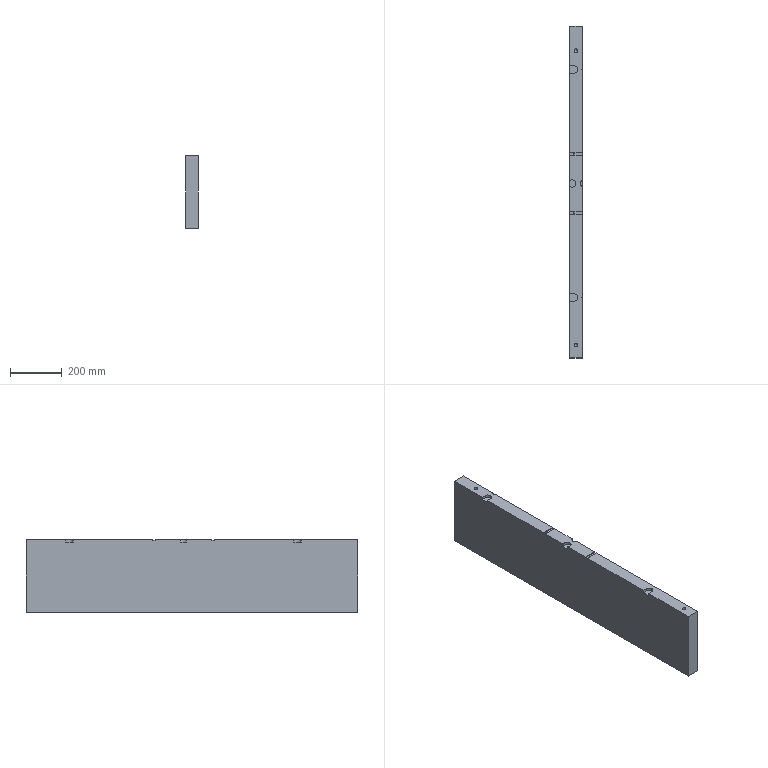Part | NX | features 29 2 | 1 solid | 44 faces | box 50 x 1280 x 280.5 mm | volume 17889049 mm3 | plane 24 | cylinder 13 | cone 7 | commonest cylinder face diameters 14.1 x5 28 x3 29 x3 3.4 x2
STEP:
#1=CARTESIAN_POINT('',(2892.05,512.5,-493.5));
#2=VERTEX_POINT('',#1);
#3=CARTESIAN_POINT('',(2885.,512.5,-493.5));
#4=DIRECTION('',(0.,0.,1.));
#5=DIRECTION('',(1.,0.,0.));
#6=AXIS2_PLACEMENT_3D('',#3,#4,#5);
#7=CIRCLE('',#6,7.05);
#8=EDGE_CURVE('',#2,#2,#7,.T.);
#9=ORIENTED_EDGE('',*,*,#8,.T.);
#10=EDGE_LOOP('',(#9));
#11=FACE_BOUND('',#10,.T.);
#12=CARTESIAN_POINT('',(2860.,607.5,-493.5));
#13=VERTEX_POINT('',#12);
#14=CARTESIAN_POINT('',(2860.,-672.5,-493.5));
#15=VERTEX_POINT('',#14);
#16=CARTESIAN_POINT('',(2860.,193.,-493.5));
#17=DIRECTION('',(0.,-1.,0.));
#18=VECTOR('',#17,1000.);
#19=LINE('',#16,#18);
#20=EDGE_CURVE('',#13,#15,#19,.T.);
#21=ORIENTED_EDGE('',*,*,#20,.F.);
#22=CARTESIAN_POINT('',(2910.,607.5,-493.5));
#23=VERTEX_POINT('',#22);
#24=CARTESIAN_POINT('',(2901.,607.5,-493.5));
#25=DIRECTION('',(1.,0.,0.));
#26=VECTOR('',#25,1000.);
#27=LINE('',#24,#26);
#28=EDGE_CURVE('',#13,#23,#27,.T.);
#29=ORIENTED_EDGE('',*,*,#28,.T.);
#30=CARTESIAN_POINT('',(2910.,-672.5,-493.5));
#31=VERTEX_POINT('',#30);
#32=CARTESIAN_POINT('',(2910.,193.,-493.5));
#33=DIRECTION('',(0.,1.,0.));
#34=VECTOR('',#33,1000.);
#35=LINE('',#32,#34);
#36=EDGE_CURVE('',#31,#23,#35,.T.);
#37=ORIENTED_EDGE('',*,*,#36,.F.);
#38=CARTESIAN_POINT('',(3250.,-672.5,-493.5));
#39=DIRECTION('',(-1.,0.,0.));
#40=VECTOR('',#39,1000.);
#41=LINE('',#38,#40);
#42=EDGE_CURVE('',#31,#15,#41,.T.);
#43=ORIENTED_EDGE('',*,*,#42,.T.);
#44=EDGE_LOOP('',(#21,#29,#37,#43));
#45=FACE_BOUND('',#44,.T.);
#46=CARTESIAN_POINT('',(2892.05,-622.5,-493.5));
#47=VERTEX_POINT('',#46);
#48=CARTESIAN_POINT('',(2885.,-622.5,-493.5));
#49=DIRECTION('',(0.,0.,1.));
#50=DIRECTION('',(1.,0.,0.));
#51=AXIS2_PLACEMENT_3D('',#48,#49,#50);
#52=CIRCLE('',#51,7.05);
#53=EDGE_CURVE('',#47,#47,#52,.T.);
#54=ORIENTED_EDGE('',*,*,#53,.T.);
#55=EDGE_LOOP('',(#54));
#56=FACE_BOUND('',#55,.T.);
#57=CARTESIAN_POINT('',(2892.05,-32.5,-493.5));
#58=VERTEX_POINT('',#57);
#59=CARTESIAN_POINT('',(2885.,-32.5,-493.5));
#60=DIRECTION('',(0.,0.,1.));
#61=DIRECTION('',(1.,0.,0.));
#62=AXIS2_PLACEMENT_3D('',#59,#60,#61);
#63=CIRCLE('',#62,7.05);
#64=EDGE_CURVE('',#58,#58,#63,.T.);
#65=ORIENTED_EDGE('',*,*,#64,.T.);
#66=EDGE_LOOP('',(#65));
#67=FACE_BOUND('',#66,.T.);
#68=CARTESIAN_POINT('',(1985.,0.,-493.5));
#69=DIRECTION('',(0.,0.,-1.));
#70=DIRECTION('',(1.,0.,0.));
#71=AXIS2_PLACEMENT_3D('',#68,#69,#70);
#72=PLANE('',#71);
#73=ADVANCED_FACE('',(#11,#45,#56,#67),#72,.T.);
#74=CARTESIAN_POINT('',(2910.,120.5,-213.));
#75=VERTEX_POINT('',#74);
#76=CARTESIAN_POINT('',(2860.,120.5,-213.));
#77=VERTEX_POINT('',#76);
#78=CARTESIAN_POINT('',(1985.,120.5,-213.));
#79=DIRECTION('',(-1.,0.,0.));
#80=VECTOR('',#79,1000.);
#81=LINE('',#78,#80);
#82=EDGE_CURVE('',#75,#77,#81,.T.);
#83=ORIENTED_EDGE('',*,*,#82,.F.);
#84=CARTESIAN_POINT('',(2910.,432.789,-213.));
#85=VERTEX_POINT('',#84);
#86=CARTESIAN_POINT('',(2910.,193.,-213.));
#87=DIRECTION('',(0.,-1.,0.));
#88=VECTOR('',#87,1000.);
#89=LINE('',#86,#88);
#90=EDGE_CURVE('',#85,#75,#89,.T.);
#91=ORIENTED_EDGE('',*,*,#90,.F.);
#92=CARTESIAN_POINT('',(2910.,447.211,-213.));
#93=VERTEX_POINT('',#92);
#94=CARTESIAN_POINT('',(2922.,440.,-213.));
#95=DIRECTION('',(0.,0.,1.));
#96=DIRECTION('',(-1.,0.,0.));
#97=AXIS2_PLACEMENT_3D('',#94,#95,#96);
#98=CIRCLE('',#97,14.);
#99=EDGE_CURVE('',#93,#85,#98,.T.);
#100=ORIENTED_EDGE('',*,*,#99,.F.);
#101=CARTESIAN_POINT('',(2910.,607.5,-213.));
#102=VERTEX_POINT('',#101);
#103=CARTESIAN_POINT('',(2910.,193.,-213.));
#104=DIRECTION('',(0.,-1.,0.));
#105=VECTOR('',#104,1000.);
#106=LINE('',#103,#105);
#107=EDGE_CURVE('',#102,#93,#106,.T.);
#108=ORIENTED_EDGE('',*,*,#107,.F.);
#109=CARTESIAN_POINT('',(2860.,607.5,-213.));
#110=VERTEX_POINT('',#109);
#111=CARTESIAN_POINT('',(2901.,607.5,-213.));
#112=DIRECTION('',(-1.,0.,0.));
#113=VECTOR('',#112,1000.);
#114=LINE('',#111,#113);
#115=EDGE_CURVE('',#102,#110,#114,.T.);
#116=ORIENTED_EDGE('',*,*,#115,.T.);
#117=CARTESIAN_POINT('',(2860.,454.5,-213.));
#118=VERTEX_POINT('',#117);
#119=CARTESIAN_POINT('',(2860.,193.,-213.));
#120=DIRECTION('',(0.,1.,0.));
#121=VECTOR('',#120,1000.);
#122=LINE('',#119,#121);
#123=EDGE_CURVE('',#118,#110,#122,.T.);
#124=ORIENTED_EDGE('',*,*,#123,.F.);
#125=CARTESIAN_POINT('',(2877.,454.5,-213.));
#126=VERTEX_POINT('',#125);
#127=CARTESIAN_POINT('',(1985.,454.5,-213.));
#128=DIRECTION('',(-1.,0.,0.));
#129=VECTOR('',#128,1000.);
#130=LINE('',#127,#129);
#131=EDGE_CURVE('',#126,#118,#130,.T.);
#132=ORIENTED_EDGE('',*,*,#131,.F.);
#133=CARTESIAN_POINT('',(2877.,425.5,-213.));
#134=VERTEX_POINT('',#133);
#135=CARTESIAN_POINT('',(2877.,440.,-213.));
#136=DIRECTION('',(0.,0.,1.));
#137=DIRECTION('',(-1.,0.,0.));
#138=AXIS2_PLACEMENT_3D('',#135,#136,#137);
#139=CIRCLE('',#138,14.5);
#140=EDGE_CURVE('',#134,#126,#139,.T.);
#141=ORIENTED_EDGE('',*,*,#140,.F.);
#142=CARTESIAN_POINT('',(2860.,425.5,-213.));
#143=VERTEX_POINT('',#142);
#144=CARTESIAN_POINT('',(1985.,425.5,-213.));
#145=DIRECTION('',(1.,0.,0.));
#146=VECTOR('',#145,1000.);
#147=LINE('',#144,#146);
#148=EDGE_CURVE('',#143,#134,#147,.T.);
#149=ORIENTED_EDGE('',*,*,#148,.F.);
#150=CARTESIAN_POINT('',(2860.,193.,-213.));
#151=DIRECTION('',(0.,1.,0.));
#152=VECTOR('',#151,1000.);
#153=LINE('',#150,#152);
#154=EDGE_CURVE('',#77,#143,#153,.T.);
#155=ORIENTED_EDGE('',*,*,#154,.F.);
#156=EDGE_LOOP('',(#83,#91,#100,#108,#116,#124,#132,#141,#149,#155));
#157=FACE_BOUND('',#156,.T.);
#158=CARTESIAN_POINT('',(2892.05,512.5,-213.));
#159=VERTEX_POINT('',#158);
#160=CARTESIAN_POINT('',(2885.,512.5,-213.));
#161=DIRECTION('',(0.,0.,-1.));
#162=DIRECTION('',(1.,0.,0.));
#163=AXIS2_PLACEMENT_3D('',#160,#161,#162);
#164=CIRCLE('',#163,7.05);
#165=EDGE_CURVE('',#159,#159,#164,.T.);
#166=ORIENTED_EDGE('',*,*,#165,.T.);
#167=EDGE_LOOP('',(#166));
#168=FACE_BOUND('',#167,.T.);
#169=CARTESIAN_POINT('',(1985.,0.,-213.));
#170=DIRECTION('',(0.,0.,1.));
#171=DIRECTION('',(-1.,0.,0.));
#172=AXIS2_PLACEMENT_3D('',#169,#170,#171);
#173=PLANE('',#172);
#174=ADVANCED_FACE('',(#157,#168),#173,.T.);
#175=CARTESIAN_POINT('',(2860.,-120.5,-213.));
#176=VERTEX_POINT('',#175);
#177=CARTESIAN_POINT('',(2910.,-120.5,-213.));
#178=VERTEX_POINT('',#177);
#179=CARTESIAN_POINT('',(1985.,-120.5,-213.));
#180=DIRECTION('',(1.,0.,0.));
#181=VECTOR('',#180,1000.);
#182=LINE('',#179,#181);
#183=EDGE_CURVE('',#176,#178,#182,.T.);
#184=ORIENTED_EDGE('',*,*,#183,.F.);
#185=CARTESIAN_POINT('',(2860.,-425.5,-213.));
#186=VERTEX_POINT('',#185);
#187=CARTESIAN_POINT('',(2860.,193.,-213.));
#188=DIRECTION('',(0.,1.,0.));
#189=VECTOR('',#188,1000.);
#190=LINE('',#187,#189);
#191=EDGE_CURVE('',#186,#176,#190,.T.);
#192=ORIENTED_EDGE('',*,*,#191,.F.);
#193=CARTESIAN_POINT('',(2877.,-425.5,-213.));
#194=VERTEX_POINT('',#193);
#195=CARTESIAN_POINT('',(1985.,-425.5,-213.));
#196=DIRECTION('',(-1.,0.,0.));
#197=VECTOR('',#196,1000.);
#198=LINE('',#195,#197);
#199=EDGE_CURVE('',#194,#186,#198,.T.);
#200=ORIENTED_EDGE('',*,*,#199,.F.);
#201=CARTESIAN_POINT('',(2877.,-454.5,-213.));
#202=VERTEX_POINT('',#201);
#203=CARTESIAN_POINT('',(2877.,-440.,-213.));
#204=DIRECTION('',(0.,0.,1.));
#205=DIRECTION('',(-1.,0.,0.));
#206=AXIS2_PLACEMENT_3D('',#203,#204,#205);
#207=CIRCLE('',#206,14.5);
#208=EDGE_CURVE('',#202,#194,#207,.T.);
#209=ORIENTED_EDGE('',*,*,#208,.F.);
#210=CARTESIAN_POINT('',(2860.,-454.5,-213.));
#211=VERTEX_POINT('',#210);
#212=CARTESIAN_POINT('',(1985.,-454.5,-213.));
#213=DIRECTION('',(1.,0.,0.));
#214=VECTOR('',#213,1000.);
#215=LINE('',#212,#214);
#216=EDGE_CURVE('',#211,#202,#215,.T.);
#217=ORIENTED_EDGE('',*,*,#216,.F.);
#218=CARTESIAN_POINT('',(2860.,-672.5,-213.));
#219=VERTEX_POINT('',#218);
#220=CARTESIAN_POINT('',(2860.,193.,-213.));
#221=DIRECTION('',(0.,1.,0.));
#222=VECTOR('',#221,1000.);
#223=LINE('',#220,#222);
#224=EDGE_CURVE('',#219,#211,#223,.T.);
#225=ORIENTED_EDGE('',*,*,#224,.F.);
#226=CARTESIAN_POINT('',(2910.,-672.5,-213.));
#227=VERTEX_POINT('',#226);
#228=CARTESIAN_POINT('',(3250.,-672.5,-213.));
#229=DIRECTION('',(1.,0.,0.));
#230=VECTOR('',#229,1000.);
#231=LINE('',#228,#230);
#232=EDGE_CURVE('',#219,#227,#231,.T.);
#233=ORIENTED_EDGE('',*,*,#232,.T.);
#234=CARTESIAN_POINT('',(2910.,-447.211,-213.));
#235=VERTEX_POINT('',#234);
#236=CARTESIAN_POINT('',(2910.,193.,-213.));
#237=DIRECTION('',(0.,-1.,0.));
#238=VECTOR('',#237,1000.);
#239=LINE('',#236,#238);
#240=EDGE_CURVE('',#235,#227,#239,.T.);
#241=ORIENTED_EDGE('',*,*,#240,.F.);
#242=CARTESIAN_POINT('',(2910.,-432.789,-213.));
#243=VERTEX_POINT('',#242);
#244=CARTESIAN_POINT('',(2922.,-440.,-213.));
#245=DIRECTION('',(0.,0.,1.));
#246=DIRECTION('',(-1.,0.,0.));
#247=AXIS2_PLACEMENT_3D('',#244,#245,#246);
#248=CIRCLE('',#247,14.);
#249=EDGE_CURVE('',#243,#235,#248,.T.);
#250=ORIENTED_EDGE('',*,*,#249,.F.);
#251=CARTESIAN_POINT('',(2910.,193.,-213.));
#252=DIRECTION('',(0.,-1.,0.));
#253=VECTOR('',#252,1000.);
#254=LINE('',#251,#253);
#255=EDGE_CURVE('',#178,#243,#254,.T.);
#256=ORIENTED_EDGE('',*,*,#255,.F.);
#257=EDGE_LOOP('',(#184,#192,#200,#209,#217,#225,#233,#241,#250,#256));
#258=FACE_BOUND('',#257,.T.);
#259=CARTESIAN_POINT('',(2892.05,-622.5,-213.));
#260=VERTEX_POINT('',#259);
#261=CARTESIAN_POINT('',(2885.,-622.5,-213.));
#262=DIRECTION('',(0.,0.,-1.));
#263=DIRECTION('',(1.,0.,0.));
#264=AXIS2_PLACEMENT_3D('',#261,#262,#263);
#265=CIRCLE('',#264,7.05);
#266=EDGE_CURVE('',#260,#260,#265,.T.);
#267=ORIENTED_EDGE('',*,*,#266,.T.);
#268=EDGE_LOOP('',(#267));
#269=FACE_BOUND('',#268,.T.);
#270=CARTESIAN_POINT('',(1985.,0.,-213.));
#271=DIRECTION('',(0.,0.,1.));
#272=DIRECTION('',(-1.,0.,0.));
#273=AXIS2_PLACEMENT_3D('',#270,#271,#272);
#274=PLANE('',#273);
#275=ADVANCED_FACE('',(#258,#269),#274,.T.);
#276=CARTESIAN_POINT('',(2910.,-109.5,-213.));
#277=VERTEX_POINT('',#276);
#278=CARTESIAN_POINT('',(2860.,-109.5,-213.));
#279=VERTEX_POINT('',#278);
#280=CARTESIAN_POINT('',(1985.,-109.5,-213.));
#281=DIRECTION('',(-1.,0.,0.));
#282=VECTOR('',#281,1000.);
#283=LINE('',#280,#282);
#284=EDGE_CURVE('',#277,#279,#283,.T.);
#285=ORIENTED_EDGE('',*,*,#284,.F.);
#286=CARTESIAN_POINT('',(2910.,-13.077,-213.));
#287=VERTEX_POINT('',#286);
#288=CARTESIAN_POINT('',(2910.,193.,-213.));
#289=DIRECTION('',(0.,-1.,0.));
#290=VECTOR('',#289,1000.);
#291=LINE('',#288,#290);
#292=EDGE_CURVE('',#287,#277,#291,.T.);
#293=ORIENTED_EDGE('',*,*,#292,.F.);
#294=CARTESIAN_POINT('',(2910.,13.077,-213.));
#295=VERTEX_POINT('',#294);
#296=CARTESIAN_POINT('',(2915.,0.,-213.));
#297=DIRECTION('',(0.,0.,1.));
#298=DIRECTION('',(-1.,0.,0.));
#299=AXIS2_PLACEMENT_3D('',#296,#297,#298);
#300=CIRCLE('',#299,14.);
#301=EDGE_CURVE('',#295,#287,#300,.T.);
#302=ORIENTED_EDGE('',*,*,#301,.F.);
#303=CARTESIAN_POINT('',(2910.,109.5,-213.));
#304=VERTEX_POINT('',#303);
#305=CARTESIAN_POINT('',(2910.,193.,-213.));
#306=DIRECTION('',(0.,-1.,0.));
#307=VECTOR('',#306,1000.);
#308=LINE('',#305,#307);
#309=EDGE_CURVE('',#304,#295,#308,.T.);
#310=ORIENTED_EDGE('',*,*,#309,.F.);
#311=CARTESIAN_POINT('',(2860.,109.5,-213.));
#312=VERTEX_POINT('',#311);
#313=CARTESIAN_POINT('',(1985.,109.5,-213.));
#314=DIRECTION('',(1.,0.,0.));
#315=VECTOR('',#314,1000.);
#316=LINE('',#313,#315);
#317=EDGE_CURVE('',#312,#304,#316,.T.);
#318=ORIENTED_EDGE('',*,*,#317,.F.);
#319=CARTESIAN_POINT('',(2860.,10.5,-213.));
#320=VERTEX_POINT('',#319);
#321=CARTESIAN_POINT('',(2860.,193.,-213.));
#322=DIRECTION('',(0.,1.,0.));
#323=VECTOR('',#322,1000.);
#324=LINE('',#321,#323);
#325=EDGE_CURVE('',#320,#312,#324,.T.);
#326=ORIENTED_EDGE('',*,*,#325,.F.);
#327=CARTESIAN_POINT('',(2860.,-10.5,-213.));
#328=VERTEX_POINT('',#327);
#329=CARTESIAN_POINT('',(2870.,0.,-213.));
#330=DIRECTION('',(0.,0.,-1.));
#331=DIRECTION('',(-1.,0.,0.));
#332=AXIS2_PLACEMENT_3D('',#329,#330,#331);
#333=CIRCLE('',#332,14.5);
#334=EDGE_CURVE('',#320,#328,#333,.T.);
#335=ORIENTED_EDGE('',*,*,#334,.T.);
#336=CARTESIAN_POINT('',(2860.,193.,-213.));
#337=DIRECTION('',(0.,1.,0.));
#338=VECTOR('',#337,1000.);
#339=LINE('',#336,#338);
#340=EDGE_CURVE('',#279,#328,#339,.T.);
#341=ORIENTED_EDGE('',*,*,#340,.F.);
#342=EDGE_LOOP('',(#285,#293,#302,#310,#318,#326,#335,#341));
#343=FACE_BOUND('',#342,.T.);
#344=CARTESIAN_POINT('',(1985.,0.,-213.));
#345=DIRECTION('',(0.,0.,1.));
#346=DIRECTION('',(-1.,0.,0.));
#347=AXIS2_PLACEMENT_3D('',#344,#345,#346);
#348=PLANE('',#347);
#349=ADVANCED_FACE('',(#343),#348,.T.);
#350=CARTESIAN_POINT('',(2877.,425.5,-223.));
#351=VERTEX_POINT('',#350);
#352=CARTESIAN_POINT('',(2877.,425.5,-193.));
#353=DIRECTION('',(0.,0.,-1.));
#354=VECTOR('',#353,1000.);
#355=LINE('',#352,#354);
#356=EDGE_CURVE('',#134,#351,#355,.T.);
#357=ORIENTED_EDGE('',*,*,#356,.F.);
#358=ORIENTED_EDGE('',*,*,#140,.T.);
#359=CARTESIAN_POINT('',(2877.,454.5,-223.));
#360=VERTEX_POINT('',#359);
#361=CARTESIAN_POINT('',(2877.,454.5,-193.));
#362=DIRECTION('',(0.,0.,1.));
#363=VECTOR('',#362,1000.);
#364=LINE('',#361,#363);
#365=EDGE_CURVE('',#360,#126,#364,.T.);
#366=ORIENTED_EDGE('',*,*,#365,.F.);
#367=CARTESIAN_POINT('',(2877.,440.,-223.));
#368=DIRECTION('',(0.,0.,-1.));
#369=DIRECTION('',(-1.,0.,0.));
#370=AXIS2_PLACEMENT_3D('',#367,#368,#369);
#371=CIRCLE('',#370,14.5);
#372=EDGE_CURVE('',#360,#351,#371,.T.);
#373=ORIENTED_EDGE('',*,*,#372,.T.);
#374=EDGE_LOOP('',(#357,#358,#366,#373));
#375=FACE_BOUND('',#374,.T.);
#376=CARTESIAN_POINT('',(2877.,440.,-223.));
#377=DIRECTION('',(0.,0.,1.));
#378=DIRECTION('',(-1.,0.,0.));
#379=AXIS2_PLACEMENT_3D('',#376,#377,#378);
#380=CYLINDRICAL_SURFACE('',#379,14.5);
#381=ADVANCED_FACE('',(#375),#380,.F.);
#382=CARTESIAN_POINT('',(2877.,-454.5,-223.));
#383=VERTEX_POINT('',#382);
#384=CARTESIAN_POINT('',(2877.,-454.5,-193.));
#385=DIRECTION('',(0.,0.,-1.));
#386=VECTOR('',#385,1000.);
#387=LINE('',#384,#386);
#388=EDGE_CURVE('',#202,#383,#387,.T.);
#389=ORIENTED_EDGE('',*,*,#388,.F.);
#390=ORIENTED_EDGE('',*,*,#208,.T.);
#391=CARTESIAN_POINT('',(2877.,-425.5,-223.));
#392=VERTEX_POINT('',#391);
#393=CARTESIAN_POINT('',(2877.,-425.5,-193.));
#394=DIRECTION('',(0.,0.,1.));
#395=VECTOR('',#394,1000.);
#396=LINE('',#393,#395);
#397=EDGE_CURVE('',#392,#194,#396,.T.);
#398=ORIENTED_EDGE('',*,*,#397,.F.);
#399=CARTESIAN_POINT('',(2877.,-440.,-223.));
#400=DIRECTION('',(0.,0.,-1.));
#401=DIRECTION('',(-1.,0.,0.));
#402=AXIS2_PLACEMENT_3D('',#399,#400,#401);
#403=CIRCLE('',#402,14.5);
#404=EDGE_CURVE('',#392,#383,#403,.T.);
#405=ORIENTED_EDGE('',*,*,#404,.T.);
#406=EDGE_LOOP('',(#389,#390,#398,#405));
#407=FACE_BOUND('',#406,.T.);
#408=CARTESIAN_POINT('',(2877.,-440.,-223.));
#409=DIRECTION('',(0.,0.,1.));
#410=DIRECTION('',(-1.,0.,0.));
#411=AXIS2_PLACEMENT_3D('',#408,#409,#410);
#412=CYLINDRICAL_SURFACE('',#411,14.5);
#413=ADVANCED_FACE('',(#407),#412,.F.);
#414=CARTESIAN_POINT('',(2860.,-109.5,-216.));
#415=VERTEX_POINT('',#414);
#416=CARTESIAN_POINT('',(2860.,-109.5,-205.5));
#417=DIRECTION('',(0.,0.,-1.));
#418=VECTOR('',#417,1000.);
#419=LINE('',#416,#418);
#420=EDGE_CURVE('',#279,#415,#419,.T.);
#421=ORIENTED_EDGE('',*,*,#420,.F.);
#422=ORIENTED_EDGE('',*,*,#340,.T.);
#423=CARTESIAN_POINT('',(2860.,-10.5,-223.));
#424=VERTEX_POINT('',#423);
#425=CARTESIAN_POINT('',(2860.,-10.5,-223.));
#426=DIRECTION('',(0.,0.,-1.));
#427=VECTOR('',#426,1000.);
#428=LINE('',#425,#427);
#429=EDGE_CURVE('',#328,#424,#428,.T.);
#430=ORIENTED_EDGE('',*,*,#429,.T.);
#431=CARTESIAN_POINT('',(2860.,10.5,-223.));
#432=VERTEX_POINT('',#431);
#433=CARTESIAN_POINT('',(2860.,193.,-223.));
#434=DIRECTION('',(0.,-1.,0.));
#435=VECTOR('',#434,1000.);
#436=LINE('',#433,#435);
#437=EDGE_CURVE('',#432,#424,#436,.T.);
#438=ORIENTED_EDGE('',*,*,#437,.F.);
#439=CARTESIAN_POINT('',(2860.,10.5,-223.));
#440=DIRECTION('',(0.,0.,1.));
#441=VECTOR('',#440,1000.);
#442=LINE('',#439,#441);
#443=EDGE_CURVE('',#432,#320,#442,.T.);
#444=ORIENTED_EDGE('',*,*,#443,.T.);
#445=ORIENTED_EDGE('',*,*,#325,.T.);
#446=CARTESIAN_POINT('',(2860.,109.5,-216.));
#447=VERTEX_POINT('',#446);
#448=CARTESIAN_POINT('',(2860.,109.5,-205.5));
#449=DIRECTION('',(0.,0.,1.));
#450=VECTOR('',#449,1000.);
#451=LINE('',#448,#450);
#452=EDGE_CURVE('',#447,#312,#451,.T.);
#453=ORIENTED_EDGE('',*,*,#452,.F.);
#454=CARTESIAN_POINT('',(2860.,120.5,-216.));
#455=VERTEX_POINT('',#454);
#456=CARTESIAN_POINT('',(2860.,193.,-216.));
#457=DIRECTION('',(0.,-1.,0.));
#458=VECTOR('',#457,1000.);
#459=LINE('',#456,#458);
#460=EDGE_CURVE('',#455,#447,#459,.T.);
#461=ORIENTED_EDGE('',*,*,#460,.F.);
#462=CARTESIAN_POINT('',(2860.,120.5,-205.5));
#463=DIRECTION('',(0.,0.,-1.));
#464=VECTOR('',#463,1000.);
#465=LINE('',#462,#464);
#466=EDGE_CURVE('',#77,#455,#465,.T.);
#467=ORIENTED_EDGE('',*,*,#466,.F.);
#468=ORIENTED_EDGE('',*,*,#154,.T.);
#469=CARTESIAN_POINT('',(2860.,425.5,-223.));
#470=VERTEX_POINT('',#469);
#471=CARTESIAN_POINT('',(2860.,425.5,-205.5));
#472=DIRECTION('',(0.,0.,1.));
#473=VECTOR('',#472,1000.);
#474=LINE('',#471,#473);
#475=EDGE_CURVE('',#470,#143,#474,.T.);
#476=ORIENTED_EDGE('',*,*,#475,.F.);
#477=CARTESIAN_POINT('',(2860.,454.5,-223.));
#478=VERTEX_POINT('',#477);
#479=CARTESIAN_POINT('',(2860.,193.,-223.));
#480=DIRECTION('',(0.,1.,0.));
#481=VECTOR('',#480,1000.);
#482=LINE('',#479,#481);
#483=EDGE_CURVE('',#470,#478,#482,.T.);
#484=ORIENTED_EDGE('',*,*,#483,.T.);
#485=CARTESIAN_POINT('',(2860.,454.5,-205.5));
#486=DIRECTION('',(0.,0.,-1.));
#487=VECTOR('',#486,1000.);
#488=LINE('',#485,#487);
#489=EDGE_CURVE('',#118,#478,#488,.T.);
#490=ORIENTED_EDGE('',*,*,#489,.F.);
#491=ORIENTED_EDGE('',*,*,#123,.T.);
#492=CARTESIAN_POINT('',(2860.,607.5,-205.5));
#493=DIRECTION('',(0.,0.,1.));
#494=VECTOR('',#493,1000.);
#495=LINE('',#492,#494);
#496=EDGE_CURVE('',#13,#110,#495,.T.);
#497=ORIENTED_EDGE('',*,*,#496,.F.);
#498=ORIENTED_EDGE('',*,*,#20,.T.);
#499=CARTESIAN_POINT('',(2860.,-672.5,-113.));
#500=DIRECTION('',(0.,0.,1.));
#501=VECTOR('',#500,1000.);
#502=LINE('',#499,#501);
#503=EDGE_CURVE('',#15,#219,#502,.T.);
#504=ORIENTED_EDGE('',*,*,#503,.T.);
#505=ORIENTED_EDGE('',*,*,#224,.T.);
#506=CARTESIAN_POINT('',(2860.,-454.5,-223.));
#507=VERTEX_POINT('',#506);
#508=CARTESIAN_POINT('',(2860.,-454.5,-205.5));
#509=DIRECTION('',(0.,0.,1.));
#510=VECTOR('',#509,1000.);
#511=LINE('',#508,#510);
#512=EDGE_CURVE('',#507,#211,#511,.T.);
#513=ORIENTED_EDGE('',*,*,#512,.F.);
#514=CARTESIAN_POINT('',(2860.,-425.5,-223.));
#515=VERTEX_POINT('',#514);
#516=CARTESIAN_POINT('',(2860.,193.,-223.));
#517=DIRECTION('',(0.,1.,0.));
#518=VECTOR('',#517,1000.);
#519=LINE('',#516,#518);
#520=EDGE_CURVE('',#507,#515,#519,.T.);
#521=ORIENTED_EDGE('',*,*,#520,.T.);
#522=CARTESIAN_POINT('',(2860.,-425.5,-205.5));
#523=DIRECTION('',(0.,0.,-1.));
#524=VECTOR('',#523,1000.);
#525=LINE('',#522,#524);
#526=EDGE_CURVE('',#186,#515,#525,.T.);
#527=ORIENTED_EDGE('',*,*,#526,.F.);
#528=ORIENTED_EDGE('',*,*,#191,.T.);
#529=CARTESIAN_POINT('',(2860.,-120.5,-216.));
#530=VERTEX_POINT('',#529);
#531=CARTESIAN_POINT('',(2860.,-120.5,-205.5));
#532=DIRECTION('',(0.,0.,1.));
#533=VECTOR('',#532,1000.);
#534=LINE('',#531,#533);
#535=EDGE_CURVE('',#530,#176,#534,.T.);
#536=ORIENTED_EDGE('',*,*,#535,.F.);
#537=CARTESIAN_POINT('',(2860.,193.,-216.));
#538=DIRECTION('',(0.,-1.,0.));
#539=VECTOR('',#538,1000.);
#540=LINE('',#537,#539);
#541=EDGE_CURVE('',#415,#530,#540,.T.);
#542=ORIENTED_EDGE('',*,*,#541,.F.);
#543=EDGE_LOOP('',(#421,#422,#430,#438,#444,#445,#453,#461,#467,#468,#476,#484,#490,#491,#497,#498,#504,#505,#513,#521,#527,#528,#536,#542));
#544=FACE_BOUND('',#543,.T.);
#545=CARTESIAN_POINT('',(2860.,193.,-205.5));
#546=DIRECTION('',(-1.,0.,0.));
#547=DIRECTION('',(0.,0.,1.));
#548=AXIS2_PLACEMENT_3D('',#545,#546,#547);
#549=PLANE('',#548);
#550=ADVANCED_FACE('',(#544),#549,.T.);
#551=ORIENTED_EDGE('',*,*,#28,.F.);
#552=ORIENTED_EDGE('',*,*,#496,.T.);
#553=ORIENTED_EDGE('',*,*,#115,.F.);
#554=CARTESIAN_POINT('',(2910.,607.5,-339.));
#555=DIRECTION('',(0.,0.,1.));
#556=VECTOR('',#555,1000.);
#557=LINE('',#554,#556);
#558=EDGE_CURVE('',#23,#102,#557,.T.);
#559=ORIENTED_EDGE('',*,*,#558,.F.);
#560=EDGE_LOOP('',(#551,#552,#553,#559));
#561=FACE_BOUND('',#560,.T.);
#562=CARTESIAN_POINT('',(2901.,607.5,-339.));
#563=DIRECTION('',(0.,1.,0.));
#564=DIRECTION('',(1.,0.,0.));
#565=AXIS2_PLACEMENT_3D('',#562,#563,#564);
#566=PLANE('',#565);
#567=ADVANCED_FACE('',(#561),#566,.T.);
#568=CARTESIAN_POINT('',(2910.,-109.5,-216.));
#569=VERTEX_POINT('',#568);
#570=CARTESIAN_POINT('',(2910.,-109.5,-205.5));
#571=DIRECTION('',(0.,0.,1.));
#572=VECTOR('',#571,1000.);
#573=LINE('',#570,#572);
#574=EDGE_CURVE('',#569,#277,#573,.T.);
#575=ORIENTED_EDGE('',*,*,#574,.F.);
#576=CARTESIAN_POINT('',(2910.,-120.5,-216.));
#577=VERTEX_POINT('',#576);
#578=CARTESIAN_POINT('',(2910.,193.,-216.));
#579=DIRECTION('',(0.,1.,0.));
#580=VECTOR('',#579,1000.);
#581=LINE('',#578,#580);
#582=EDGE_CURVE('',#577,#569,#581,.T.);
#583=ORIENTED_EDGE('',*,*,#582,.F.);
#584=CARTESIAN_POINT('',(2910.,-120.5,-205.5));
#585=DIRECTION('',(0.,0.,-1.));
#586=VECTOR('',#585,1000.);
#587=LINE('',#584,#586);
#588=EDGE_CURVE('',#178,#577,#587,.T.);
#589=ORIENTED_EDGE('',*,*,#588,.F.);
#590=ORIENTED_EDGE('',*,*,#255,.T.);
#591=CARTESIAN_POINT('',(2910.,-432.789,-243.));
#592=VERTEX_POINT('',#591);
#593=CARTESIAN_POINT('',(2910.,-432.789,-243.));
#594=DIRECTION('',(0.,0.,1.));
#595=VECTOR('',#594,1000.);
#596=LINE('',#593,#595);
#597=EDGE_CURVE('',#592,#243,#596,.T.);
#598=ORIENTED_EDGE('',*,*,#597,.F.);
#599=CARTESIAN_POINT('',(2910.,-447.211,-243.));
#600=VERTEX_POINT('',#599);
#601=CARTESIAN_POINT('',(2910.,193.,-243.));
#602=DIRECTION('',(0.,-1.,0.));
#603=VECTOR('',#602,1000.);
#604=LINE('',#601,#603);
#605=EDGE_CURVE('',#592,#600,#604,.T.);
#606=ORIENTED_EDGE('',*,*,#605,.T.);
#607=CARTESIAN_POINT('',(2910.,-447.211,-243.));
#608=DIRECTION('',(0.,0.,-1.));
#609=VECTOR('',#608,1000.);
#610=LINE('',#607,#609);
#611=EDGE_CURVE('',#235,#600,#610,.T.);
#612=ORIENTED_EDGE('',*,*,#611,.F.);
#613=ORIENTED_EDGE('',*,*,#240,.T.);
#614=CARTESIAN_POINT('',(2910.,-672.5,-543.5));
#615=DIRECTION('',(0.,0.,1.));
#616=VECTOR('',#615,1000.);
#617=LINE('',#614,#616);
#618=EDGE_CURVE('',#31,#227,#617,.T.);
#619=ORIENTED_EDGE('',*,*,#618,.F.);
#620=ORIENTED_EDGE('',*,*,#36,.T.);
#621=ORIENTED_EDGE('',*,*,#558,.T.);
#622=ORIENTED_EDGE('',*,*,#107,.T.);
#623=CARTESIAN_POINT('',(2910.,447.211,-243.));
#624=VERTEX_POINT('',#623);
#625=CARTESIAN_POINT('',(2910.,447.211,-243.));
#626=DIRECTION('',(0.,0.,1.));
#627=VECTOR('',#626,1000.);
#628=LINE('',#625,#627);
#629=EDGE_CURVE('',#624,#93,#628,.T.);
#630=ORIENTED_EDGE('',*,*,#629,.F.);
#631=CARTESIAN_POINT('',(2910.,432.789,-243.));
#632=VERTEX_POINT('',#631);
#633=CARTESIAN_POINT('',(2910.,193.,-243.));
#634=DIRECTION('',(0.,-1.,0.));
#635=VECTOR('',#634,1000.);
#636=LINE('',#633,#635);
#637=EDGE_CURVE('',#624,#632,#636,.T.);
#638=ORIENTED_EDGE('',*,*,#637,.T.);
#639=CARTESIAN_POINT('',(2910.,432.789,-243.));
#640=DIRECTION('',(0.,0.,-1.));
#641=VECTOR('',#640,1000.);
#642=LINE('',#639,#641);
#643=EDGE_CURVE('',#85,#632,#642,.T.);
#644=ORIENTED_EDGE('',*,*,#643,.F.);
#645=ORIENTED_EDGE('',*,*,#90,.T.);
#646=CARTESIAN_POINT('',(2910.,120.5,-216.));
#647=VERTEX_POINT('',#646);
#648=CARTESIAN_POINT('',(2910.,120.5,-205.5));
#649=DIRECTION('',(0.,0.,1.));
#650=VECTOR('',#649,1000.);
#651=LINE('',#648,#650);
#652=EDGE_CURVE('',#647,#75,#651,.T.);
#653=ORIENTED_EDGE('',*,*,#652,.F.);
#654=CARTESIAN_POINT('',(2910.,109.5,-216.));
#655=VERTEX_POINT('',#654);
#656=CARTESIAN_POINT('',(2910.,193.,-216.));
#657=DIRECTION('',(0.,1.,0.));
#658=VECTOR('',#657,1000.);
#659=LINE('',#656,#658);
#660=EDGE_CURVE('',#655,#647,#659,.T.);
#661=ORIENTED_EDGE('',*,*,#660,.F.);
#662=CARTESIAN_POINT('',(2910.,109.5,-205.5));
#663=DIRECTION('',(0.,0.,-1.));
#664=VECTOR('',#663,1000.);
#665=LINE('',#662,#664);
#666=EDGE_CURVE('',#304,#655,#665,.T.);
#667=ORIENTED_EDGE('',*,*,#666,.F.);
#668=ORIENTED_EDGE('',*,*,#309,.T.);
#669=CARTESIAN_POINT('',(2910.,13.077,-243.));
#670=VERTEX_POINT('',#669);
#671=CARTESIAN_POINT('',(2910.,13.077,-243.));
#672=DIRECTION('',(0.,0.,1.));
#673=VECTOR('',#672,1000.);
#674=LINE('',#671,#673);
#675=EDGE_CURVE('',#670,#295,#674,.T.);
#676=ORIENTED_EDGE('',*,*,#675,.F.);
#677=CARTESIAN_POINT('',(2910.,-13.077,-243.));
#678=VERTEX_POINT('',#677);
#679=CARTESIAN_POINT('',(2910.,193.,-243.));
#680=DIRECTION('',(0.,-1.,0.));
#681=VECTOR('',#680,1000.);
#682=LINE('',#679,#681);
#683=EDGE_CURVE('',#670,#678,#682,.T.);
#684=ORIENTED_EDGE('',*,*,#683,.T.);
#685=CARTESIAN_POINT('',(2910.,-13.077,-243.));
#686=DIRECTION('',(0.,0.,-1.));
#687=VECTOR('',#686,1000.);
#688=LINE('',#685,#687);
#689=EDGE_CURVE('',#287,#678,#688,.T.);
#690=ORIENTED_EDGE('',*,*,#689,.F.);
#691=ORIENTED_EDGE('',*,*,#292,.T.);
#692=EDGE_LOOP('',(#575,#583,#589,#590,#598,#606,#612,#613,#619,#620,#621,#622,#630,#638,#644,#645,#653,#661,#667,#668,#676,#684,#690,#691));
#693=FACE_BOUND('',#692,.T.);
#694=CARTESIAN_POINT('',(2910.,193.,-205.5));
#695=DIRECTION('',(1.,0.,0.));
#696=DIRECTION('',(0.,0.,-1.));
#697=AXIS2_PLACEMENT_3D('',#694,#695,#696);
#698=PLANE('',#697);
#699=ADVANCED_FACE('',(#693),#698,.T.);
#700=ORIENTED_EDGE('',*,*,#42,.F.);
#701=ORIENTED_EDGE('',*,*,#618,.T.);
#702=ORIENTED_EDGE('',*,*,#232,.F.);
#703=ORIENTED_EDGE('',*,*,#503,.F.);
#704=EDGE_LOOP('',(#700,#701,#702,#703));
#705=FACE_BOUND('',#704,.T.);
#706=CARTESIAN_POINT('',(3250.,-672.5,-113.));
#707=DIRECTION('',(0.,1.,0.));
#708=DIRECTION('',(1.,0.,0.));
#709=AXIS2_PLACEMENT_3D('',#706,#707,#708);
#710=PLANE('',#709);
#711=ADVANCED_FACE('',(#705),#710,.F.);
#712=ORIENTED_EDGE('',*,*,#597,.T.);
#713=ORIENTED_EDGE('',*,*,#249,.T.);
#714=ORIENTED_EDGE('',*,*,#611,.T.);
#715=CARTESIAN_POINT('',(2922.,-440.,-243.));
#716=DIRECTION('',(0.,0.,-1.));
#717=DIRECTION('',(-1.,0.,0.));
#718=AXIS2_PLACEMENT_3D('',#715,#716,#717);
#719=CIRCLE('',#718,14.);
#720=EDGE_CURVE('',#600,#592,#719,.T.);
#721=ORIENTED_EDGE('',*,*,#720,.T.);
#722=EDGE_LOOP('',(#712,#713,#714,#721));
#723=FACE_BOUND('',#722,.T.);
#724=CARTESIAN_POINT('',(2922.,-440.,-243.));
#725=DIRECTION('',(0.,0.,1.));
#726=DIRECTION('',(-1.,0.,0.));
#727=AXIS2_PLACEMENT_3D('',#724,#725,#726);
#728=CYLINDRICAL_SURFACE('',#727,14.);
#729=ADVANCED_FACE('',(#723),#728,.F.);
#730=ORIENTED_EDGE('',*,*,#720,.F.);
#731=ORIENTED_EDGE('',*,*,#605,.F.);
#732=EDGE_LOOP('',(#730,#731));
#733=FACE_BOUND('',#732,.T.);
#734=CARTESIAN_POINT('',(2922.,-440.,-243.));
#735=DIRECTION('',(0.,0.,1.));
#736=DIRECTION('',(-1.,0.,0.));
#737=AXIS2_PLACEMENT_3D('',#734,#735,#736);
#738=PLANE('',#737);
#739=ADVANCED_FACE('',(#733),#738,.T.);
#740=ORIENTED_EDGE('',*,*,#675,.T.);
#741=ORIENTED_EDGE('',*,*,#301,.T.);
#742=ORIENTED_EDGE('',*,*,#689,.T.);
#743=CARTESIAN_POINT('',(2915.,0.,-243.));
#744=DIRECTION('',(0.,0.,-1.));
#745=DIRECTION('',(-1.,0.,0.));
#746=AXIS2_PLACEMENT_3D('',#743,#744,#745);
#747=CIRCLE('',#746,14.);
#748=EDGE_CURVE('',#678,#670,#747,.T.);
#749=ORIENTED_EDGE('',*,*,#748,.T.);
#750=EDGE_LOOP('',(#740,#741,#742,#749));
#751=FACE_BOUND('',#750,.T.);
#752=CARTESIAN_POINT('',(2915.,0.,-243.));
#753=DIRECTION('',(0.,0.,1.));
#754=DIRECTION('',(-1.,0.,0.));
#755=AXIS2_PLACEMENT_3D('',#752,#753,#754);
#756=CYLINDRICAL_SURFACE('',#755,14.);
#757=ADVANCED_FACE('',(#751),#756,.F.);
#758=ORIENTED_EDGE('',*,*,#748,.F.);
#759=ORIENTED_EDGE('',*,*,#683,.F.);
#760=EDGE_LOOP('',(#758,#759));
#761=FACE_BOUND('',#760,.T.);
#762=CARTESIAN_POINT('',(2915.,0.,-243.));
#763=DIRECTION('',(0.,0.,1.));
#764=DIRECTION('',(-1.,0.,0.));
#765=AXIS2_PLACEMENT_3D('',#762,#763,#764);
#766=PLANE('',#765);
#767=ADVANCED_FACE('',(#761),#766,.T.);
#768=ORIENTED_EDGE('',*,*,#629,.T.);
#769=ORIENTED_EDGE('',*,*,#99,.T.);
#770=ORIENTED_EDGE('',*,*,#643,.T.);
#771=CARTESIAN_POINT('',(2922.,440.,-243.));
#772=DIRECTION('',(0.,0.,-1.));
#773=DIRECTION('',(-1.,0.,0.));
#774=AXIS2_PLACEMENT_3D('',#771,#772,#773);
#775=CIRCLE('',#774,14.);
#776=EDGE_CURVE('',#632,#624,#775,.T.);
#777=ORIENTED_EDGE('',*,*,#776,.T.);
#778=EDGE_LOOP('',(#768,#769,#770,#777));
#779=FACE_BOUND('',#778,.T.);
#780=CARTESIAN_POINT('',(2922.,440.,-243.));
#781=DIRECTION('',(0.,0.,1.));
#782=DIRECTION('',(-1.,0.,0.));
#783=AXIS2_PLACEMENT_3D('',#780,#781,#782);
#784=CYLINDRICAL_SURFACE('',#783,14.);
#785=ADVANCED_FACE('',(#779),#784,.F.);
#786=ORIENTED_EDGE('',*,*,#776,.F.);
#787=ORIENTED_EDGE('',*,*,#637,.F.);
#788=EDGE_LOOP('',(#786,#787));
#789=FACE_BOUND('',#788,.T.);
#790=CARTESIAN_POINT('',(2922.,440.,-243.));
#791=DIRECTION('',(0.,0.,1.));
#792=DIRECTION('',(-1.,0.,0.));
#793=AXIS2_PLACEMENT_3D('',#790,#791,#792);
#794=PLANE('',#793);
#795=ADVANCED_FACE('',(#789),#794,.T.);
#796=ORIENTED_EDGE('',*,*,#334,.F.);
#797=ORIENTED_EDGE('',*,*,#443,.F.);
#798=CARTESIAN_POINT('',(2870.,0.,-223.));
#799=DIRECTION('',(0.,0.,1.));
#800=DIRECTION('',(-1.,0.,0.));
#801=AXIS2_PLACEMENT_3D('',#798,#799,#800);
#802=CIRCLE('',#801,14.5);
#803=EDGE_CURVE('',#424,#432,#802,.T.);
#804=ORIENTED_EDGE('',*,*,#803,.F.);
#805=ORIENTED_EDGE('',*,*,#429,.F.);
#806=EDGE_LOOP('',(#796,#797,#804,#805));
#807=FACE_BOUND('',#806,.T.);
#808=CARTESIAN_POINT('',(2870.,0.,-223.));
#809=DIRECTION('',(0.,0.,1.));
#810=DIRECTION('',(-1.,0.,0.));
#811=AXIS2_PLACEMENT_3D('',#808,#809,#810);
#812=CYLINDRICAL_SURFACE('',#811,14.5);
#813=ADVANCED_FACE('',(#807),#812,.F.);
#814=ORIENTED_EDGE('',*,*,#437,.T.);
#815=ORIENTED_EDGE('',*,*,#803,.T.);
#816=EDGE_LOOP('',(#814,#815));
#817=FACE_BOUND('',#816,.T.);
#818=CARTESIAN_POINT('',(2870.,0.,-223.));
#819=DIRECTION('',(0.,0.,-1.));
#820=DIRECTION('',(1.,0.,0.));
#821=AXIS2_PLACEMENT_3D('',#818,#819,#820);
#822=PLANE('',#821);
#823=ADVANCED_FACE('',(#817),#822,.F.);
#824=ORIENTED_EDGE('',*,*,#404,.F.);
#825=CARTESIAN_POINT('',(2847.,-425.5,-223.));
#826=DIRECTION('',(1.,0.,0.));
#827=VECTOR('',#826,1000.);
#828=LINE('',#825,#827);
#829=EDGE_CURVE('',#515,#392,#828,.T.);
#830=ORIENTED_EDGE('',*,*,#829,.F.);
#831=ORIENTED_EDGE('',*,*,#520,.F.);
#832=CARTESIAN_POINT('',(2847.,-454.5,-223.));
#833=DIRECTION('',(1.,0.,0.));
#834=VECTOR('',#833,1000.);
#835=LINE('',#832,#834);
#836=EDGE_CURVE('',#507,#383,#835,.T.);
#837=ORIENTED_EDGE('',*,*,#836,.T.);
#838=EDGE_LOOP('',(#824,#830,#831,#837));
#839=FACE_BOUND('',#838,.T.);
#840=CARTESIAN_POINT('',(2877.,-440.,-223.));
#841=DIRECTION('',(0.,0.,1.));
#842=DIRECTION('',(-1.,0.,0.));
#843=AXIS2_PLACEMENT_3D('',#840,#841,#842);
#844=PLANE('',#843);
#845=ADVANCED_FACE('',(#839),#844,.T.);
#846=ORIENTED_EDGE('',*,*,#372,.F.);
#847=CARTESIAN_POINT('',(2847.,454.5,-223.));
#848=DIRECTION('',(1.,0.,0.));
#849=VECTOR('',#848,1000.);
#850=LINE('',#847,#849);
#851=EDGE_CURVE('',#478,#360,#850,.T.);
#852=ORIENTED_EDGE('',*,*,#851,.F.);
#853=ORIENTED_EDGE('',*,*,#483,.F.);
#854=CARTESIAN_POINT('',(2847.,425.5,-223.));
#855=DIRECTION('',(1.,0.,0.));
#856=VECTOR('',#855,1000.);
#857=LINE('',#854,#856);
#858=EDGE_CURVE('',#470,#351,#857,.T.);
#859=ORIENTED_EDGE('',*,*,#858,.T.);
#860=EDGE_LOOP('',(#846,#852,#853,#859));
#861=FACE_BOUND('',#860,.T.);
#862=CARTESIAN_POINT('',(2877.,440.,-223.));
#863=DIRECTION('',(0.,0.,1.));
#864=DIRECTION('',(-1.,0.,0.));
#865=AXIS2_PLACEMENT_3D('',#862,#863,#864);
#866=PLANE('',#865);
#867=ADVANCED_FACE('',(#861),#866,.T.);
#868=ORIENTED_EDGE('',*,*,#526,.T.);
#869=ORIENTED_EDGE('',*,*,#829,.T.);
#870=ORIENTED_EDGE('',*,*,#397,.T.);
#871=ORIENTED_EDGE('',*,*,#199,.T.);
#872=EDGE_LOOP('',(#868,#869,#870,#871));
#873=FACE_BOUND('',#872,.T.);
#874=CARTESIAN_POINT('',(2847.,-425.5,-193.));
#875=DIRECTION('',(0.,1.,0.));
#876=DIRECTION('',(0.,0.,-1.));
#877=AXIS2_PLACEMENT_3D('',#874,#875,#876);
#878=PLANE('',#877);
#879=ADVANCED_FACE('',(#873),#878,.F.);
#880=ORIENTED_EDGE('',*,*,#512,.T.);
#881=ORIENTED_EDGE('',*,*,#216,.T.);
#882=ORIENTED_EDGE('',*,*,#388,.T.);
#883=ORIENTED_EDGE('',*,*,#836,.F.);
#884=EDGE_LOOP('',(#880,#881,#882,#883));
#885=FACE_BOUND('',#884,.T.);
#886=CARTESIAN_POINT('',(2847.,-454.5,-193.));
#887=DIRECTION('',(0.,-1.,0.));
#888=DIRECTION('',(0.,0.,1.));
#889=AXIS2_PLACEMENT_3D('',#886,#887,#888);
#890=PLANE('',#889);
#891=ADVANCED_FACE('',(#885),#890,.F.);
#892=ORIENTED_EDGE('',*,*,#489,.T.);
#893=ORIENTED_EDGE('',*,*,#851,.T.);
#894=ORIENTED_EDGE('',*,*,#365,.T.);
#895=ORIENTED_EDGE('',*,*,#131,.T.);
#896=EDGE_LOOP('',(#892,#893,#894,#895));
#897=FACE_BOUND('',#896,.T.);
#898=CARTESIAN_POINT('',(2847.,454.5,-193.));
#899=DIRECTION('',(0.,1.,0.));
#900=DIRECTION('',(0.,0.,-1.));
#901=AXIS2_PLACEMENT_3D('',#898,#899,#900);
#902=PLANE('',#901);
#903=ADVANCED_FACE('',(#897),#902,.F.);
#904=ORIENTED_EDGE('',*,*,#475,.T.);
#905=ORIENTED_EDGE('',*,*,#148,.T.);
#906=ORIENTED_EDGE('',*,*,#356,.T.);
#907=ORIENTED_EDGE('',*,*,#858,.F.);
#908=EDGE_LOOP('',(#904,#905,#906,#907));
#909=FACE_BOUND('',#908,.T.);
#910=CARTESIAN_POINT('',(2847.,425.5,-193.));
#911=DIRECTION('',(0.,-1.,0.));
#912=DIRECTION('',(0.,0.,1.));
#913=AXIS2_PLACEMENT_3D('',#910,#911,#912);
#914=PLANE('',#913);
#915=ADVANCED_FACE('',(#909),#914,.F.);
#916=ORIENTED_EDGE('',*,*,#452,.T.);
#917=ORIENTED_EDGE('',*,*,#317,.T.);
#918=ORIENTED_EDGE('',*,*,#666,.T.);
#919=CARTESIAN_POINT('',(2881.,109.5,-216.));
#920=DIRECTION('',(-1.,0.,0.));
#921=VECTOR('',#920,1000.);
#922=LINE('',#919,#921);
#923=EDGE_CURVE('',#655,#447,#922,.T.);
#924=ORIENTED_EDGE('',*,*,#923,.T.);
#925=EDGE_LOOP('',(#916,#917,#918,#924));
#926=FACE_BOUND('',#925,.T.);
#927=CARTESIAN_POINT('',(2881.,109.5,-216.));
#928=DIRECTION('',(0.,-1.,0.));
#929=DIRECTION('',(0.,0.,1.));
#930=AXIS2_PLACEMENT_3D('',#927,#928,#929);
#931=PLANE('',#930);
#932=ADVANCED_FACE('',(#926),#931,.F.);
#933=ORIENTED_EDGE('',*,*,#466,.T.);
#934=CARTESIAN_POINT('',(2881.,120.5,-216.));
#935=DIRECTION('',(1.,0.,0.));
#936=VECTOR('',#935,1000.);
#937=LINE('',#934,#936);
#938=EDGE_CURVE('',#455,#647,#937,.T.);
#939=ORIENTED_EDGE('',*,*,#938,.T.);
#940=ORIENTED_EDGE('',*,*,#652,.T.);
#941=ORIENTED_EDGE('',*,*,#82,.T.);
#942=EDGE_LOOP('',(#933,#939,#940,#941));
#943=FACE_BOUND('',#942,.T.);
#944=CARTESIAN_POINT('',(2881.,120.5,-216.));
#945=DIRECTION('',(0.,1.,0.));
#946=DIRECTION('',(0.,0.,-1.));
#947=AXIS2_PLACEMENT_3D('',#944,#945,#946);
#948=PLANE('',#947);
#949=ADVANCED_FACE('',(#943),#948,.F.);
#950=CARTESIAN_POINT('',(2874.3,115.,-216.));
#951=VERTEX_POINT('',#950);
#952=CARTESIAN_POINT('',(2876.,115.,-216.));
#953=DIRECTION('',(0.,0.,-1.));
#954=DIRECTION('',(-1.,0.,0.));
#955=AXIS2_PLACEMENT_3D('',#952,#953,#954);
#956=CIRCLE('',#955,1.7);
#957=EDGE_CURVE('',#951,#951,#956,.T.);
#958=ORIENTED_EDGE('',*,*,#957,.T.);
#959=EDGE_LOOP('',(#958));
#960=FACE_BOUND('',#959,.T.);
#961=ORIENTED_EDGE('',*,*,#460,.T.);
#962=ORIENTED_EDGE('',*,*,#923,.F.);
#963=ORIENTED_EDGE('',*,*,#660,.T.);
#964=ORIENTED_EDGE('',*,*,#938,.F.);
#965=EDGE_LOOP('',(#961,#962,#963,#964));
#966=FACE_BOUND('',#965,.T.);
#967=CARTESIAN_POINT('',(2881.,115.,-216.));
#968=DIRECTION('',(0.,0.,-1.));
#969=DIRECTION('',(1.,0.,0.));
#970=AXIS2_PLACEMENT_3D('',#967,#968,#969);
#971=PLANE('',#970);
#972=ADVANCED_FACE('',(#960,#966),#971,.F.);
#973=ORIENTED_EDGE('',*,*,#420,.T.);
#974=CARTESIAN_POINT('',(2881.,-109.5,-216.));
#975=DIRECTION('',(-1.,0.,0.));
#976=VECTOR('',#975,1000.);
#977=LINE('',#974,#976);
#978=EDGE_CURVE('',#569,#415,#977,.T.);
#979=ORIENTED_EDGE('',*,*,#978,.F.);
#980=ORIENTED_EDGE('',*,*,#574,.T.);
#981=ORIENTED_EDGE('',*,*,#284,.T.);
#982=EDGE_LOOP('',(#973,#979,#980,#981));
#983=FACE_BOUND('',#982,.T.);
#984=CARTESIAN_POINT('',(2881.,-109.5,-216.));
#985=DIRECTION('',(0.,1.,0.));
#986=DIRECTION('',(0.,0.,1.));
#987=AXIS2_PLACEMENT_3D('',#984,#985,#986);
#988=PLANE('',#987);
#989=ADVANCED_FACE('',(#983),#988,.F.);
#990=ORIENTED_EDGE('',*,*,#535,.T.);
#991=ORIENTED_EDGE('',*,*,#183,.T.);
#992=ORIENTED_EDGE('',*,*,#588,.T.);
#993=CARTESIAN_POINT('',(2881.,-120.5,-216.));
#994=DIRECTION('',(1.,0.,0.));
#995=VECTOR('',#994,1000.);
#996=LINE('',#993,#995);
#997=EDGE_CURVE('',#530,#577,#996,.T.);
#998=ORIENTED_EDGE('',*,*,#997,.F.);
#999=EDGE_LOOP('',(#990,#991,#992,#998));
#1000=FACE_BOUND('',#999,.T.);
#1001=CARTESIAN_POINT('',(2881.,-120.5,-216.));
#1002=DIRECTION('',(0.,-1.,0.));
#1003=DIRECTION('',(0.,0.,-1.));
#1004=AXIS2_PLACEMENT_3D('',#1001,#1002,#1003);
#1005=PLANE('',#1004);
#1006=ADVANCED_FACE('',(#1000),#1005,.F.);
#1007=CARTESIAN_POINT('',(2874.3,-115.,-216.));
#1008=VERTEX_POINT('',#1007);
#1009=CARTESIAN_POINT('',(2876.,-115.,-216.));
#1010=DIRECTION('',(0.,0.,-1.));
#1011=DIRECTION('',(-1.,0.,0.));
#1012=AXIS2_PLACEMENT_3D('',#1009,#1010,#1011);
#1013=CIRCLE('',#1012,1.7);
#1014=EDGE_CURVE('',#1008,#1008,#1013,.T.);
#1015=ORIENTED_EDGE('',*,*,#1014,.T.);
#1016=EDGE_LOOP('',(#1015));
#1017=FACE_BOUND('',#1016,.T.);
#1018=ORIENTED_EDGE('',*,*,#541,.T.);
#1019=ORIENTED_EDGE('',*,*,#997,.T.);
#1020=ORIENTED_EDGE('',*,*,#582,.T.);
#1021=ORIENTED_EDGE('',*,*,#978,.T.);
#1022=EDGE_LOOP('',(#1018,#1019,#1020,#1021));
#1023=FACE_BOUND('',#1022,.T.);
#1024=CARTESIAN_POINT('',(2881.,-115.,-216.));
#1025=DIRECTION('',(0.,0.,-1.));
#1026=DIRECTION('',(1.,0.,0.));
#1027=AXIS2_PLACEMENT_3D('',#1024,#1025,#1026);
#1028=PLANE('',#1027);
#1029=ADVANCED_FACE('',(#1017,#1023),#1028,.F.);
#1030=CARTESIAN_POINT('',(2877.95,-622.5,-249.95));
#1031=VERTEX_POINT('',#1030);
#1032=CARTESIAN_POINT('',(2885.,-622.5,-249.95));
#1033=DIRECTION('',(0.,0.,-1.));
#1034=DIRECTION('',(-1.,0.,0.));
#1035=AXIS2_PLACEMENT_3D('',#1032,#1033,#1034);
#1036=CIRCLE('',#1035,7.05);
#1037=EDGE_CURVE('',#1031,#1031,#1036,.T.);
#1038=ORIENTED_EDGE('',*,*,#1037,.T.);
#1039=EDGE_LOOP('',(#1038));
#1040=FACE_BOUND('',#1039,.T.);
#1041=ORIENTED_EDGE('',*,*,#266,.F.);
#1042=EDGE_LOOP('',(#1041));
#1043=FACE_BOUND('',#1042,.T.);
#1044=CARTESIAN_POINT('',(2885.,-622.5,-213.));
#1045=DIRECTION('',(0.,0.,-1.));
#1046=DIRECTION('',(-1.,0.,0.));
#1047=AXIS2_PLACEMENT_3D('',#1044,#1045,#1046);
#1048=CYLINDRICAL_SURFACE('',#1047,7.05);
#1049=ADVANCED_FACE('',(#1040,#1043),#1048,.F.);
#1050=CARTESIAN_POINT('',(2885.,-622.5,-257.));
#1051=VERTEX_POINT('',#1050);
#1052=VERTEX_LOOP('',#1051);
#1053=FACE_BOUND('',#1052,.T.);
#1054=ORIENTED_EDGE('',*,*,#1037,.F.);
#1055=EDGE_LOOP('',(#1054));
#1056=FACE_BOUND('',#1055,.T.);
#1057=CARTESIAN_POINT('',(2885.,-622.5,-249.95));
#1058=DIRECTION('',(0.,0.,1.));
#1059=DIRECTION('',(-1.,0.,0.));
#1060=AXIS2_PLACEMENT_3D('',#1057,#1058,#1059);
#1061=CONICAL_SURFACE('',#1060,7.05,0.7854);
#1062=ADVANCED_FACE('',(#1053,#1056),#1061,.F.);
#1063=CARTESIAN_POINT('',(2877.95,512.5,-249.95));
#1064=VERTEX_POINT('',#1063);
#1065=CARTESIAN_POINT('',(2885.,512.5,-249.95));
#1066=DIRECTION('',(0.,0.,-1.));
#1067=DIRECTION('',(-1.,0.,0.));
#1068=AXIS2_PLACEMENT_3D('',#1065,#1066,#1067);
#1069=CIRCLE('',#1068,7.05);
#1070=EDGE_CURVE('',#1064,#1064,#1069,.T.);
#1071=ORIENTED_EDGE('',*,*,#1070,.T.);
#1072=EDGE_LOOP('',(#1071));
#1073=FACE_BOUND('',#1072,.T.);
#1074=ORIENTED_EDGE('',*,*,#165,.F.);
#1075=EDGE_LOOP('',(#1074));
#1076=FACE_BOUND('',#1075,.T.);
#1077=CARTESIAN_POINT('',(2885.,512.5,-213.));
#1078=DIRECTION('',(0.,0.,-1.));
#1079=DIRECTION('',(-1.,0.,0.));
#1080=AXIS2_PLACEMENT_3D('',#1077,#1078,#1079);
#1081=CYLINDRICAL_SURFACE('',#1080,7.05);
#1082=ADVANCED_FACE('',(#1073,#1076),#1081,.F.);
#1083=CARTESIAN_POINT('',(2885.,512.5,-257.));
#1084=VERTEX_POINT('',#1083);
#1085=VERTEX_LOOP('',#1084);
#1086=FACE_BOUND('',#1085,.T.);
#1087=ORIENTED_EDGE('',*,*,#1070,.F.);
#1088=EDGE_LOOP('',(#1087));
#1089=FACE_BOUND('',#1088,.T.);
#1090=CARTESIAN_POINT('',(2885.,512.5,-249.95));
#1091=DIRECTION('',(0.,0.,1.));
#1092=DIRECTION('',(-1.,0.,0.));
#1093=AXIS2_PLACEMENT_3D('',#1090,#1091,#1092);
#1094=CONICAL_SURFACE('',#1093,7.05,0.7854);
#1095=ADVANCED_FACE('',(#1086,#1089),#1094,.F.);
#1096=CARTESIAN_POINT('',(2874.3,-115.,-229.3));
#1097=VERTEX_POINT('',#1096);
#1098=CARTESIAN_POINT('',(2876.,-115.,-229.3));
#1099=DIRECTION('',(0.,0.,-1.));
#1100=DIRECTION('',(-1.,0.,0.));
#1101=AXIS2_PLACEMENT_3D('',#1098,#1099,#1100);
#1102=CIRCLE('',#1101,1.7);
#1103=EDGE_CURVE('',#1097,#1097,#1102,.T.);
#1104=ORIENTED_EDGE('',*,*,#1103,.T.);
#1105=EDGE_LOOP('',(#1104));
#1106=FACE_BOUND('',#1105,.T.);
#1107=ORIENTED_EDGE('',*,*,#1014,.F.);
#1108=EDGE_LOOP('',(#1107));
#1109=FACE_BOUND('',#1108,.T.);
#1110=CARTESIAN_POINT('',(2876.,-115.,-213.));
#1111=DIRECTION('',(0.,0.,-1.));
#1112=DIRECTION('',(-1.,0.,0.));
#1113=AXIS2_PLACEMENT_3D('',#1110,#1111,#1112);
#1114=CYLINDRICAL_SURFACE('',#1113,1.7);
#1115=ADVANCED_FACE('',(#1106,#1109),#1114,.F.);
#1116=CARTESIAN_POINT('',(2876.,-115.,-231.));
#1117=VERTEX_POINT('',#1116);
#1118=VERTEX_LOOP('',#1117);
#1119=FACE_BOUND('',#1118,.T.);
#1120=ORIENTED_EDGE('',*,*,#1103,.F.);
#1121=EDGE_LOOP('',(#1120));
#1122=FACE_BOUND('',#1121,.T.);
#1123=CARTESIAN_POINT('',(2876.,-115.,-229.3));
#1124=DIRECTION('',(0.,0.,1.));
#1125=DIRECTION('',(-1.,0.,0.));
#1126=AXIS2_PLACEMENT_3D('',#1123,#1124,#1125);
#1127=CONICAL_SURFACE('',#1126,1.7,0.7854);
#1128=ADVANCED_FACE('',(#1119,#1122),#1127,.F.);
#1129=CARTESIAN_POINT('',(2874.3,115.,-229.3));
#1130=VERTEX_POINT('',#1129);
#1131=CARTESIAN_POINT('',(2876.,115.,-229.3));
#1132=DIRECTION('',(0.,0.,-1.));
#1133=DIRECTION('',(-1.,0.,0.));
#1134=AXIS2_PLACEMENT_3D('',#1131,#1132,#1133);
#1135=CIRCLE('',#1134,1.7);
#1136=EDGE_CURVE('',#1130,#1130,#1135,.T.);
#1137=ORIENTED_EDGE('',*,*,#1136,.T.);
#1138=EDGE_LOOP('',(#1137));
#1139=FACE_BOUND('',#1138,.T.);
#1140=ORIENTED_EDGE('',*,*,#957,.F.);
#1141=EDGE_LOOP('',(#1140));
#1142=FACE_BOUND('',#1141,.T.);
#1143=CARTESIAN_POINT('',(2876.,115.,-213.));
#1144=DIRECTION('',(0.,0.,-1.));
#1145=DIRECTION('',(-1.,0.,0.));
#1146=AXIS2_PLACEMENT_3D('',#1143,#1144,#1145);
#1147=CYLINDRICAL_SURFACE('',#1146,1.7);
#1148=ADVANCED_FACE('',(#1139,#1142),#1147,.F.);
#1149=CARTESIAN_POINT('',(2876.,115.,-231.));
#1150=VERTEX_POINT('',#1149);
#1151=VERTEX_LOOP('',#1150);
#1152=FACE_BOUND('',#1151,.T.);
#1153=ORIENTED_EDGE('',*,*,#1136,.F.);
#1154=EDGE_LOOP('',(#1153));
#1155=FACE_BOUND('',#1154,.T.);
#1156=CARTESIAN_POINT('',(2876.,115.,-229.3));
#1157=DIRECTION('',(0.,0.,1.));
#1158=DIRECTION('',(-1.,0.,0.));
#1159=AXIS2_PLACEMENT_3D('',#1156,#1157,#1158);
#1160=CONICAL_SURFACE('',#1159,1.7,0.7854);
#1161=ADVANCED_FACE('',(#1152,#1155),#1160,.F.);
#1162=CARTESIAN_POINT('',(2892.05,-622.5,-456.55));
#1163=VERTEX_POINT('',#1162);
#1164=CARTESIAN_POINT('',(2885.,-622.5,-456.55));
#1165=DIRECTION('',(0.,0.,1.));
#1166=DIRECTION('',(1.,0.,0.));
#1167=AXIS2_PLACEMENT_3D('',#1164,#1165,#1166);
#1168=CIRCLE('',#1167,7.05);
#1169=EDGE_CURVE('',#1163,#1163,#1168,.T.);
#1170=ORIENTED_EDGE('',*,*,#1169,.T.);
#1171=EDGE_LOOP('',(#1170));
#1172=FACE_BOUND('',#1171,.T.);
#1173=ORIENTED_EDGE('',*,*,#53,.F.);
#1174=EDGE_LOOP('',(#1173));
#1175=FACE_BOUND('',#1174,.T.);
#1176=CARTESIAN_POINT('',(2885.,-622.5,-493.5));
#1177=DIRECTION('',(0.,0.,1.));
#1178=DIRECTION('',(-1.,0.,0.));
#1179=AXIS2_PLACEMENT_3D('',#1176,#1177,#1178);
#1180=CYLINDRICAL_SURFACE('',#1179,7.05);
#1181=ADVANCED_FACE('',(#1172,#1175),#1180,.F.);
#1182=CARTESIAN_POINT('',(2885.,-622.5,-449.5));
#1183=VERTEX_POINT('',#1182);
#1184=VERTEX_LOOP('',#1183);
#1185=FACE_BOUND('',#1184,.T.);
#1186=ORIENTED_EDGE('',*,*,#1169,.F.);
#1187=EDGE_LOOP('',(#1186));
#1188=FACE_BOUND('',#1187,.T.);
#1189=CARTESIAN_POINT('',(2885.,-622.5,-456.55));
#1190=DIRECTION('',(0.,0.,-1.));
#1191=DIRECTION('',(1.,0.,0.));
#1192=AXIS2_PLACEMENT_3D('',#1189,#1190,#1191);
#1193=CONICAL_SURFACE('',#1192,7.05,0.7854);
#1194=ADVANCED_FACE('',(#1185,#1188),#1193,.F.);
#1195=CARTESIAN_POINT('',(2892.05,512.5,-456.55));
#1196=VERTEX_POINT('',#1195);
#1197=CARTESIAN_POINT('',(2885.,512.5,-456.55));
#1198=DIRECTION('',(0.,0.,1.));
#1199=DIRECTION('',(1.,0.,0.));
#1200=AXIS2_PLACEMENT_3D('',#1197,#1198,#1199);
#1201=CIRCLE('',#1200,7.05);
#1202=EDGE_CURVE('',#1196,#1196,#1201,.T.);
#1203=ORIENTED_EDGE('',*,*,#1202,.T.);
#1204=EDGE_LOOP('',(#1203));
#1205=FACE_BOUND('',#1204,.T.);
#1206=ORIENTED_EDGE('',*,*,#8,.F.);
#1207=EDGE_LOOP('',(#1206));
#1208=FACE_BOUND('',#1207,.T.);
#1209=CARTESIAN_POINT('',(2885.,512.5,-493.5));
#1210=DIRECTION('',(0.,0.,1.));
#1211=DIRECTION('',(-1.,0.,0.));
#1212=AXIS2_PLACEMENT_3D('',#1209,#1210,#1211);
#1213=CYLINDRICAL_SURFACE('',#1212,7.05);
#1214=ADVANCED_FACE('',(#1205,#1208),#1213,.F.);
#1215=CARTESIAN_POINT('',(2885.,512.5,-449.5));
#1216=VERTEX_POINT('',#1215);
#1217=VERTEX_LOOP('',#1216);
#1218=FACE_BOUND('',#1217,.T.);
#1219=ORIENTED_EDGE('',*,*,#1202,.F.);
#1220=EDGE_LOOP('',(#1219));
#1221=FACE_BOUND('',#1220,.T.);
#1222=CARTESIAN_POINT('',(2885.,512.5,-456.55));
#1223=DIRECTION('',(0.,0.,-1.));
#1224=DIRECTION('',(1.,0.,0.));
#1225=AXIS2_PLACEMENT_3D('',#1222,#1223,#1224);
#1226=CONICAL_SURFACE('',#1225,7.05,0.7854);
#1227=ADVANCED_FACE('',(#1218,#1221),#1226,.F.);
#1228=CARTESIAN_POINT('',(2892.05,-32.5,-456.55));
#1229=VERTEX_POINT('',#1228);
#1230=CARTESIAN_POINT('',(2885.,-32.5,-456.55));
#1231=DIRECTION('',(0.,0.,1.));
#1232=DIRECTION('',(1.,0.,0.));
#1233=AXIS2_PLACEMENT_3D('',#1230,#1231,#1232);
#1234=CIRCLE('',#1233,7.05);
#1235=EDGE_CURVE('',#1229,#1229,#1234,.T.);
#1236=ORIENTED_EDGE('',*,*,#1235,.T.);
#1237=EDGE_LOOP('',(#1236));
#1238=FACE_BOUND('',#1237,.T.);
#1239=ORIENTED_EDGE('',*,*,#64,.F.);
#1240=EDGE_LOOP('',(#1239));
#1241=FACE_BOUND('',#1240,.T.);
#1242=CARTESIAN_POINT('',(2885.,-32.5,-493.5));
#1243=DIRECTION('',(0.,0.,1.));
#1244=DIRECTION('',(-1.,0.,0.));
#1245=AXIS2_PLACEMENT_3D('',#1242,#1243,#1244);
#1246=CYLINDRICAL_SURFACE('',#1245,7.05);
#1247=ADVANCED_FACE('',(#1238,#1241),#1246,.F.);
#1248=CARTESIAN_POINT('',(2885.,-32.5,-449.5));
#1249=VERTEX_POINT('',#1248);
#1250=VERTEX_LOOP('',#1249);
#1251=FACE_BOUND('',#1250,.T.);
#1252=ORIENTED_EDGE('',*,*,#1235,.F.);
#1253=EDGE_LOOP('',(#1252));
#1254=FACE_BOUND('',#1253,.T.);
#1255=CARTESIAN_POINT('',(2885.,-32.5,-456.55));
#1256=DIRECTION('',(0.,0.,-1.));
#1257=DIRECTION('',(1.,0.,0.));
#1258=AXIS2_PLACEMENT_3D('',#1255,#1256,#1257);
#1259=CONICAL_SURFACE('',#1258,7.05,0.7854);
#1260=ADVANCED_FACE('',(#1251,#1254),#1259,.F.);
#1261=CLOSED_SHELL('',(#73,#174,#275,#349,#381,#413,#550,#567,#699,#711,#729,#739,#757,#767,#785,#795,#813,#823,#845,#867,#879,#891,#903,#915,#932,#949,#972,#989,#1006,#1029,#1049,#1062,#1082,#1095,#1115,#1128,#1148,#1161,#1181,#1194,#1214,#1227,#1247,#1260));
#1262=MANIFOLD_SOLID_BREP('',#1261);
#1263=(LENGTH_UNIT()NAMED_UNIT(*)SI_UNIT(.MILLI.,.METRE.));
#1264=UNCERTAINTY_MEASURE_WITH_UNIT(LENGTH_MEASURE(0.00001),#1263,'','');
#1265=(NAMED_UNIT(*)PLANE_ANGLE_UNIT()SI_UNIT($,.RADIAN.));
#1266=(NAMED_UNIT(*)SI_UNIT($,.STERADIAN.)SOLID_ANGLE_UNIT());
#1267=(GEOMETRIC_REPRESENTATION_CONTEXT(3)GLOBAL_UNCERTAINTY_ASSIGNED_CONTEXT((#1264))GLOBAL_UNIT_ASSIGNED_CONTEXT((#1263,#1265,#1266))REPRESENTATION_CONTEXT('',''));
#1268=ADVANCED_BREP_SHAPE_REPRESENTATION('',(#1262),#1267);